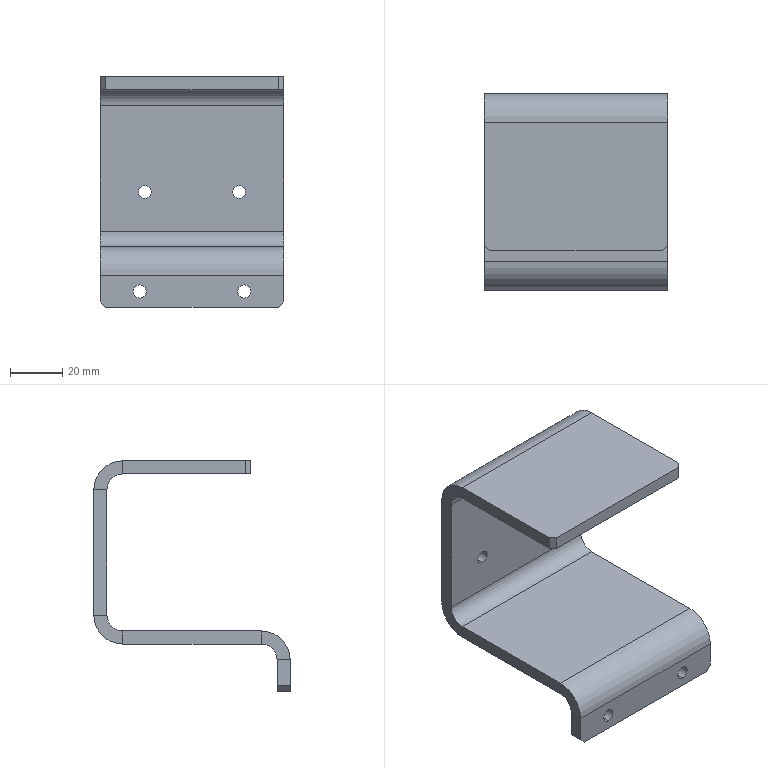Part | SolidWorks | features EdgeFlange 3, HoleWzd 2, Chamfer 1, FlatPattern 1, SMBaseFlange 1, SheetMetal 1 | 1 solid | 42 faces | box 70 x 75 x 88 mm | volume 70287 mm3 | plane 28 | cylinder 14 | commonest cylinder face diameters 5 x8 12 x3 22 x3
STEP:
#1=CARTESIAN_POINT('',(-20.,-45.,-84.5));
#2=VERTEX_POINT('',#1);
#3=CARTESIAN_POINT('',(-20.,-45.,-79.5));
#4=VERTEX_POINT('',#3);
#5=CARTESIAN_POINT('',(-20.,-45.,-82.));
#6=DIRECTION('',(0.,1.,0.));
#7=DIRECTION('',(0.,0.,1.));
#8=AXIS2_PLACEMENT_3D('',#5,#6,#7);
#9=CIRCLE('',#8,2.5);
#10=EDGE_CURVE('',#2,#4,#9,.T.);
#11=ORIENTED_EDGE('',*,*,#10,.F.);
#12=CARTESIAN_POINT('',(-20.,-40.,-84.5));
#13=VERTEX_POINT('',#12);
#14=CARTESIAN_POINT('',(-20.,-40.,-84.5));
#15=DIRECTION('',(0.,1.,0.));
#16=VECTOR('',#15,1000.);
#17=LINE('',#14,#16);
#18=EDGE_CURVE('',#2,#13,#17,.T.);
#19=ORIENTED_EDGE('',*,*,#18,.T.);
#20=CARTESIAN_POINT('',(-20.,-40.,-79.5));
#21=VERTEX_POINT('',#20);
#22=CARTESIAN_POINT('',(-20.,-40.,-82.));
#23=DIRECTION('',(0.,1.,0.));
#24=DIRECTION('',(0.,0.,1.));
#25=AXIS2_PLACEMENT_3D('',#22,#23,#24);
#26=CIRCLE('',#25,2.5);
#27=EDGE_CURVE('',#13,#21,#26,.T.);
#28=ORIENTED_EDGE('',*,*,#27,.T.);
#29=CARTESIAN_POINT('',(-20.,-40.,-79.5));
#30=DIRECTION('',(0.,1.,0.));
#31=VECTOR('',#30,1000.);
#32=LINE('',#29,#31);
#33=EDGE_CURVE('',#4,#21,#32,.T.);
#34=ORIENTED_EDGE('',*,*,#33,.F.);
#35=EDGE_LOOP('',(#11,#19,#28,#34));
#36=FACE_OUTER_BOUND('',#35,.T.);
#37=CARTESIAN_POINT('',(-20.,-40.,-82.));
#38=DIRECTION('',(0.,1.,0.));
#39=DIRECTION('',(0.,0.,1.));
#40=AXIS2_PLACEMENT_3D('',#37,#38,#39);
#41=CYLINDRICAL_SURFACE('',#40,2.5);
#42=ADVANCED_FACE('',(#36),#41,.F.);
#43=CARTESIAN_POINT('',(20.,-45.,-84.5));
#44=VERTEX_POINT('',#43);
#45=CARTESIAN_POINT('',(20.,-45.,-79.5));
#46=VERTEX_POINT('',#45);
#47=CARTESIAN_POINT('',(20.,-45.,-82.));
#48=DIRECTION('',(0.,1.,0.));
#49=DIRECTION('',(0.,0.,1.));
#50=AXIS2_PLACEMENT_3D('',#47,#48,#49);
#51=CIRCLE('',#50,2.5);
#52=EDGE_CURVE('',#44,#46,#51,.T.);
#53=ORIENTED_EDGE('',*,*,#52,.F.);
#54=CARTESIAN_POINT('',(20.,-40.,-84.5));
#55=VERTEX_POINT('',#54);
#56=CARTESIAN_POINT('',(20.,-40.,-84.5));
#57=DIRECTION('',(0.,1.,0.));
#58=VECTOR('',#57,1000.);
#59=LINE('',#56,#58);
#60=EDGE_CURVE('',#44,#55,#59,.T.);
#61=ORIENTED_EDGE('',*,*,#60,.T.);
#62=CARTESIAN_POINT('',(20.,-40.,-79.5));
#63=VERTEX_POINT('',#62);
#64=CARTESIAN_POINT('',(20.,-40.,-82.));
#65=DIRECTION('',(0.,1.,0.));
#66=DIRECTION('',(0.,0.,1.));
#67=AXIS2_PLACEMENT_3D('',#64,#65,#66);
#68=CIRCLE('',#67,2.5);
#69=EDGE_CURVE('',#55,#63,#68,.T.);
#70=ORIENTED_EDGE('',*,*,#69,.T.);
#71=CARTESIAN_POINT('',(20.,-40.,-79.5));
#72=DIRECTION('',(0.,1.,0.));
#73=VECTOR('',#72,1000.);
#74=LINE('',#71,#73);
#75=EDGE_CURVE('',#46,#63,#74,.T.);
#76=ORIENTED_EDGE('',*,*,#75,.F.);
#77=EDGE_LOOP('',(#53,#61,#70,#76));
#78=FACE_OUTER_BOUND('',#77,.T.);
#79=CARTESIAN_POINT('',(20.,-40.,-82.));
#80=DIRECTION('',(0.,1.,0.));
#81=DIRECTION('',(0.,0.,1.));
#82=AXIS2_PLACEMENT_3D('',#79,#80,#81);
#83=CYLINDRICAL_SURFACE('',#82,2.5);
#84=ADVANCED_FACE('',(#78),#83,.F.);
#85=CARTESIAN_POINT('',(-18.,25.,-46.5));
#86=VERTEX_POINT('',#85);
#87=CARTESIAN_POINT('',(-18.,25.,-41.5));
#88=VERTEX_POINT('',#87);
#89=CARTESIAN_POINT('',(-18.,25.,-44.));
#90=DIRECTION('',(0.,1.,0.));
#91=DIRECTION('',(0.,0.,1.));
#92=AXIS2_PLACEMENT_3D('',#89,#90,#91);
#93=CIRCLE('',#92,2.5);
#94=EDGE_CURVE('',#86,#88,#93,.T.);
#95=ORIENTED_EDGE('',*,*,#94,.F.);
#96=CARTESIAN_POINT('',(-18.,30.,-46.5));
#97=VERTEX_POINT('',#96);
#98=CARTESIAN_POINT('',(-18.,30.,-46.5));
#99=DIRECTION('',(0.,1.,0.));
#100=VECTOR('',#99,1000.);
#101=LINE('',#98,#100);
#102=EDGE_CURVE('',#86,#97,#101,.T.);
#103=ORIENTED_EDGE('',*,*,#102,.T.);
#104=CARTESIAN_POINT('',(-18.,30.,-41.5));
#105=VERTEX_POINT('',#104);
#106=CARTESIAN_POINT('',(-18.,30.,-44.));
#107=DIRECTION('',(0.,1.,0.));
#108=DIRECTION('',(0.,0.,1.));
#109=AXIS2_PLACEMENT_3D('',#106,#107,#108);
#110=CIRCLE('',#109,2.5);
#111=EDGE_CURVE('',#97,#105,#110,.T.);
#112=ORIENTED_EDGE('',*,*,#111,.T.);
#113=CARTESIAN_POINT('',(-18.,30.,-41.5));
#114=DIRECTION('',(0.,1.,0.));
#115=VECTOR('',#114,1000.);
#116=LINE('',#113,#115);
#117=EDGE_CURVE('',#88,#105,#116,.T.);
#118=ORIENTED_EDGE('',*,*,#117,.F.);
#119=EDGE_LOOP('',(#95,#103,#112,#118));
#120=FACE_OUTER_BOUND('',#119,.T.);
#121=CARTESIAN_POINT('',(-18.,30.,-44.));
#122=DIRECTION('',(0.,1.,0.));
#123=DIRECTION('',(0.,0.,1.));
#124=AXIS2_PLACEMENT_3D('',#121,#122,#123);
#125=CYLINDRICAL_SURFACE('',#124,2.5);
#126=ADVANCED_FACE('',(#120),#125,.F.);
#127=CARTESIAN_POINT('',(18.,25.,-46.5));
#128=VERTEX_POINT('',#127);
#129=CARTESIAN_POINT('',(18.,25.,-41.5));
#130=VERTEX_POINT('',#129);
#131=CARTESIAN_POINT('',(18.,25.,-44.));
#132=DIRECTION('',(0.,1.,0.));
#133=DIRECTION('',(0.,0.,1.));
#134=AXIS2_PLACEMENT_3D('',#131,#132,#133);
#135=CIRCLE('',#134,2.5);
#136=EDGE_CURVE('',#128,#130,#135,.T.);
#137=ORIENTED_EDGE('',*,*,#136,.F.);
#138=CARTESIAN_POINT('',(18.,30.,-46.5));
#139=VERTEX_POINT('',#138);
#140=CARTESIAN_POINT('',(18.,30.,-46.5));
#141=DIRECTION('',(0.,1.,0.));
#142=VECTOR('',#141,1000.);
#143=LINE('',#140,#142);
#144=EDGE_CURVE('',#128,#139,#143,.T.);
#145=ORIENTED_EDGE('',*,*,#144,.T.);
#146=CARTESIAN_POINT('',(18.,30.,-41.5));
#147=VERTEX_POINT('',#146);
#148=CARTESIAN_POINT('',(18.,30.,-44.));
#149=DIRECTION('',(0.,1.,0.));
#150=DIRECTION('',(0.,0.,1.));
#151=AXIS2_PLACEMENT_3D('',#148,#149,#150);
#152=CIRCLE('',#151,2.5);
#153=EDGE_CURVE('',#139,#147,#152,.T.);
#154=ORIENTED_EDGE('',*,*,#153,.T.);
#155=CARTESIAN_POINT('',(18.,30.,-41.5));
#156=DIRECTION('',(0.,1.,0.));
#157=VECTOR('',#156,1000.);
#158=LINE('',#155,#157);
#159=EDGE_CURVE('',#130,#147,#158,.T.);
#160=ORIENTED_EDGE('',*,*,#159,.F.);
#161=EDGE_LOOP('',(#137,#145,#154,#160));
#162=FACE_OUTER_BOUND('',#161,.T.);
#163=CARTESIAN_POINT('',(18.,30.,-44.));
#164=DIRECTION('',(0.,1.,0.));
#165=DIRECTION('',(0.,0.,1.));
#166=AXIS2_PLACEMENT_3D('',#163,#164,#165);
#167=CYLINDRICAL_SURFACE('',#166,2.5);
#168=ADVANCED_FACE('',(#162),#167,.F.);
#169=CARTESIAN_POINT('',(-35.,19.,-70.));
#170=VERTEX_POINT('',#169);
#171=CARTESIAN_POINT('',(-35.,-34.,-70.));
#172=VERTEX_POINT('',#171);
#173=CARTESIAN_POINT('',(-35.,-45.,-70.));
#174=DIRECTION('',(0.,-1.,0.));
#175=VECTOR('',#174,1000.);
#176=LINE('',#173,#175);
#177=EDGE_CURVE('',#170,#172,#176,.T.);
#178=ORIENTED_EDGE('',*,*,#177,.T.);
#179=CARTESIAN_POINT('',(-35.,-34.,-65.));
#180=VERTEX_POINT('',#179);
#181=CARTESIAN_POINT('',(-35.,-34.,-70.));
#182=DIRECTION('',(0.,0.,1.));
#183=VECTOR('',#182,1000.);
#184=LINE('',#181,#183);
#185=EDGE_CURVE('',#172,#180,#184,.T.);
#186=ORIENTED_EDGE('',*,*,#185,.T.);
#187=CARTESIAN_POINT('',(-35.,19.,-65.));
#188=VERTEX_POINT('',#187);
#189=CARTESIAN_POINT('',(-35.,0.,-65.));
#190=DIRECTION('',(0.,-1.,0.));
#191=VECTOR('',#190,1000.);
#192=LINE('',#189,#191);
#193=EDGE_CURVE('',#188,#180,#192,.T.);
#194=ORIENTED_EDGE('',*,*,#193,.F.);
#195=CARTESIAN_POINT('',(-35.,19.,-70.));
#196=DIRECTION('',(0.,0.,-1.));
#197=VECTOR('',#196,1000.);
#198=LINE('',#195,#197);
#199=EDGE_CURVE('',#188,#170,#198,.T.);
#200=ORIENTED_EDGE('',*,*,#199,.T.);
#201=EDGE_LOOP('',(#178,#186,#194,#200));
#202=FACE_OUTER_BOUND('',#201,.T.);
#203=CARTESIAN_POINT('',(-35.,-45.,-70.));
#204=DIRECTION('',(-1.,0.,0.));
#205=DIRECTION('',(0.,0.,1.));
#206=AXIS2_PLACEMENT_3D('',#203,#204,#205);
#207=PLANE('',#206);
#208=ADVANCED_FACE('',(#202),#207,.T.);
#209=CARTESIAN_POINT('',(35.,-34.,-70.));
#210=VERTEX_POINT('',#209);
#211=CARTESIAN_POINT('',(35.,19.,-70.));
#212=VERTEX_POINT('',#211);
#213=CARTESIAN_POINT('',(35.,25.,-70.));
#214=DIRECTION('',(0.,1.,0.));
#215=VECTOR('',#214,1000.);
#216=LINE('',#213,#215);
#217=EDGE_CURVE('',#210,#212,#216,.T.);
#218=ORIENTED_EDGE('',*,*,#217,.F.);
#219=CARTESIAN_POINT('',(-35.,-34.,-70.));
#220=DIRECTION('',(1.,0.,0.));
#221=VECTOR('',#220,1000.);
#222=LINE('',#219,#221);
#223=EDGE_CURVE('',#172,#210,#222,.T.);
#224=ORIENTED_EDGE('',*,*,#223,.F.);
#225=ORIENTED_EDGE('',*,*,#177,.F.);
#226=CARTESIAN_POINT('',(0.,19.,-70.));
#227=DIRECTION('',(1.,0.,0.));
#228=VECTOR('',#227,1000.);
#229=LINE('',#226,#228);
#230=EDGE_CURVE('',#170,#212,#229,.T.);
#231=ORIENTED_EDGE('',*,*,#230,.T.);
#232=EDGE_LOOP('',(#218,#224,#225,#231));
#233=FACE_OUTER_BOUND('',#232,.T.);
#234=CARTESIAN_POINT('',(0.,0.,-70.));
#235=DIRECTION('',(0.,0.,-1.));
#236=DIRECTION('',(0.,1.,0.));
#237=AXIS2_PLACEMENT_3D('',#234,#235,#236);
#238=PLANE('',#237);
#239=ADVANCED_FACE('',(#233),#238,.T.);
#240=CARTESIAN_POINT('',(35.,-34.,-65.));
#241=VERTEX_POINT('',#240);
#242=CARTESIAN_POINT('',(-35.,-34.,-65.));
#243=DIRECTION('',(1.,0.,0.));
#244=VECTOR('',#243,1000.);
#245=LINE('',#242,#244);
#246=EDGE_CURVE('',#180,#241,#245,.T.);
#247=ORIENTED_EDGE('',*,*,#246,.T.);
#248=CARTESIAN_POINT('',(35.,19.,-65.));
#249=VERTEX_POINT('',#248);
#250=CARTESIAN_POINT('',(35.,0.,-65.));
#251=DIRECTION('',(0.,1.,0.));
#252=VECTOR('',#251,1000.);
#253=LINE('',#250,#252);
#254=EDGE_CURVE('',#241,#249,#253,.T.);
#255=ORIENTED_EDGE('',*,*,#254,.T.);
#256=CARTESIAN_POINT('',(-35.,19.,-65.));
#257=DIRECTION('',(1.,0.,0.));
#258=VECTOR('',#257,1000.);
#259=LINE('',#256,#258);
#260=EDGE_CURVE('',#188,#249,#259,.T.);
#261=ORIENTED_EDGE('',*,*,#260,.F.);
#262=ORIENTED_EDGE('',*,*,#193,.T.);
#263=EDGE_LOOP('',(#247,#255,#261,#262));
#264=FACE_OUTER_BOUND('',#263,.T.);
#265=CARTESIAN_POINT('',(0.,0.,-65.));
#266=DIRECTION('',(0.,0.,-1.));
#267=DIRECTION('',(0.,1.,0.));
#268=AXIS2_PLACEMENT_3D('',#265,#266,#267);
#269=PLANE('',#268);
#270=ADVANCED_FACE('',(#264),#269,.F.);
#271=CARTESIAN_POINT('',(35.,25.,-59.));
#272=VERTEX_POINT('',#271);
#273=CARTESIAN_POINT('',(35.,25.,-11.));
#274=VERTEX_POINT('',#273);
#275=CARTESIAN_POINT('',(35.,25.,0.));
#276=DIRECTION('',(0.,0.,1.));
#277=VECTOR('',#276,1000.);
#278=LINE('',#275,#277);
#279=EDGE_CURVE('',#272,#274,#278,.T.);
#280=ORIENTED_EDGE('',*,*,#279,.F.);
#281=CARTESIAN_POINT('',(35.,30.,-59.));
#282=VERTEX_POINT('',#281);
#283=CARTESIAN_POINT('',(35.,25.,-59.));
#284=DIRECTION('',(0.,1.,0.));
#285=VECTOR('',#284,1000.);
#286=LINE('',#283,#285);
#287=EDGE_CURVE('',#272,#282,#286,.T.);
#288=ORIENTED_EDGE('',*,*,#287,.T.);
#289=CARTESIAN_POINT('',(35.,30.,-11.));
#290=VERTEX_POINT('',#289);
#291=CARTESIAN_POINT('',(35.,30.,-5.));
#292=DIRECTION('',(0.,0.,1.));
#293=VECTOR('',#292,1000.);
#294=LINE('',#291,#293);
#295=EDGE_CURVE('',#282,#290,#294,.T.);
#296=ORIENTED_EDGE('',*,*,#295,.T.);
#297=CARTESIAN_POINT('',(35.,25.,-11.));
#298=DIRECTION('',(0.,1.,0.));
#299=VECTOR('',#298,1000.);
#300=LINE('',#297,#299);
#301=EDGE_CURVE('',#274,#290,#300,.T.);
#302=ORIENTED_EDGE('',*,*,#301,.F.);
#303=EDGE_LOOP('',(#280,#288,#296,#302));
#304=FACE_OUTER_BOUND('',#303,.T.);
#305=CARTESIAN_POINT('',(35.,30.,-5.));
#306=DIRECTION('',(1.,0.,0.));
#307=DIRECTION('',(0.,0.,-1.));
#308=AXIS2_PLACEMENT_3D('',#305,#306,#307);
#309=PLANE('',#308);
#310=ADVANCED_FACE('',(#304),#309,.T.);
#311=CARTESIAN_POINT('',(-18.,30.,-44.));
#312=DIRECTION('',(0.,1.,0.));
#313=DIRECTION('',(0.,0.,1.));
#314=AXIS2_PLACEMENT_3D('',#311,#312,#313);
#315=CIRCLE('',#314,2.5);
#316=EDGE_CURVE('',#105,#97,#315,.T.);
#317=ORIENTED_EDGE('',*,*,#316,.F.);
#318=ORIENTED_EDGE('',*,*,#111,.F.);
#319=EDGE_LOOP('',(#317,#318));
#320=FACE_BOUND('',#319,.T.);
#321=CARTESIAN_POINT('',(18.,30.,-44.));
#322=DIRECTION('',(0.,1.,0.));
#323=DIRECTION('',(0.,0.,1.));
#324=AXIS2_PLACEMENT_3D('',#321,#322,#323);
#325=CIRCLE('',#324,2.5);
#326=EDGE_CURVE('',#147,#139,#325,.T.);
#327=ORIENTED_EDGE('',*,*,#326,.F.);
#328=ORIENTED_EDGE('',*,*,#153,.F.);
#329=EDGE_LOOP('',(#327,#328));
#330=FACE_BOUND('',#329,.T.);
#331=ORIENTED_EDGE('',*,*,#295,.F.);
#332=CARTESIAN_POINT('',(-35.,30.,-59.));
#333=VERTEX_POINT('',#332);
#334=CARTESIAN_POINT('',(35.,30.,-59.));
#335=DIRECTION('',(-1.,0.,0.));
#336=VECTOR('',#335,1000.);
#337=LINE('',#334,#336);
#338=EDGE_CURVE('',#282,#333,#337,.T.);
#339=ORIENTED_EDGE('',*,*,#338,.T.);
#340=CARTESIAN_POINT('',(-35.,30.,-11.));
#341=VERTEX_POINT('',#340);
#342=CARTESIAN_POINT('',(-35.,30.,-70.));
#343=DIRECTION('',(0.,0.,-1.));
#344=VECTOR('',#343,1000.);
#345=LINE('',#342,#344);
#346=EDGE_CURVE('',#341,#333,#345,.T.);
#347=ORIENTED_EDGE('',*,*,#346,.F.);
#348=CARTESIAN_POINT('',(0.,30.,-11.));
#349=DIRECTION('',(1.,0.,0.));
#350=VECTOR('',#349,1000.);
#351=LINE('',#348,#350);
#352=EDGE_CURVE('',#341,#290,#351,.T.);
#353=ORIENTED_EDGE('',*,*,#352,.T.);
#354=EDGE_LOOP('',(#331,#339,#347,#353));
#355=FACE_OUTER_BOUND('',#354,.T.);
#356=CARTESIAN_POINT('',(0.,30.,0.));
#357=DIRECTION('',(0.,1.,0.));
#358=DIRECTION('',(0.,0.,1.));
#359=AXIS2_PLACEMENT_3D('',#356,#357,#358);
#360=PLANE('',#359);
#361=ADVANCED_FACE('',(#320,#330,#355),#360,.T.);
#362=CARTESIAN_POINT('',(-18.,25.,-44.));
#363=DIRECTION('',(0.,1.,0.));
#364=DIRECTION('',(0.,0.,1.));
#365=AXIS2_PLACEMENT_3D('',#362,#363,#364);
#366=CIRCLE('',#365,2.5);
#367=EDGE_CURVE('',#88,#86,#366,.T.);
#368=ORIENTED_EDGE('',*,*,#367,.T.);
#369=ORIENTED_EDGE('',*,*,#94,.T.);
#370=EDGE_LOOP('',(#368,#369));
#371=FACE_BOUND('',#370,.T.);
#372=CARTESIAN_POINT('',(18.,25.,-44.));
#373=DIRECTION('',(0.,1.,0.));
#374=DIRECTION('',(0.,0.,1.));
#375=AXIS2_PLACEMENT_3D('',#372,#373,#374);
#376=CIRCLE('',#375,2.5);
#377=EDGE_CURVE('',#130,#128,#376,.T.);
#378=ORIENTED_EDGE('',*,*,#377,.T.);
#379=ORIENTED_EDGE('',*,*,#136,.T.);
#380=EDGE_LOOP('',(#378,#379));
#381=FACE_BOUND('',#380,.T.);
#382=CARTESIAN_POINT('',(-35.,25.,-59.));
#383=VERTEX_POINT('',#382);
#384=CARTESIAN_POINT('',(35.,25.,-59.));
#385=DIRECTION('',(-1.,0.,0.));
#386=VECTOR('',#385,1000.);
#387=LINE('',#384,#386);
#388=EDGE_CURVE('',#272,#383,#387,.T.);
#389=ORIENTED_EDGE('',*,*,#388,.F.);
#390=ORIENTED_EDGE('',*,*,#279,.T.);
#391=CARTESIAN_POINT('',(-35.,25.,-11.));
#392=VERTEX_POINT('',#391);
#393=CARTESIAN_POINT('',(-35.,25.,-11.));
#394=DIRECTION('',(1.,0.,0.));
#395=VECTOR('',#394,1000.);
#396=LINE('',#393,#395);
#397=EDGE_CURVE('',#392,#274,#396,.T.);
#398=ORIENTED_EDGE('',*,*,#397,.F.);
#399=CARTESIAN_POINT('',(-35.,25.,0.));
#400=DIRECTION('',(0.,0.,-1.));
#401=VECTOR('',#400,1000.);
#402=LINE('',#399,#401);
#403=EDGE_CURVE('',#392,#383,#402,.T.);
#404=ORIENTED_EDGE('',*,*,#403,.T.);
#405=EDGE_LOOP('',(#389,#390,#398,#404));
#406=FACE_OUTER_BOUND('',#405,.T.);
#407=CARTESIAN_POINT('',(0.,25.,0.));
#408=DIRECTION('',(0.,1.,0.));
#409=DIRECTION('',(0.,0.,1.));
#410=AXIS2_PLACEMENT_3D('',#407,#408,#409);
#411=PLANE('',#410);
#412=ADVANCED_FACE('',(#371,#381,#406),#411,.F.);
#413=CARTESIAN_POINT('',(35.,-28.,0.));
#414=VERTEX_POINT('',#413);
#415=CARTESIAN_POINT('',(35.,19.,0.));
#416=VERTEX_POINT('',#415);
#417=CARTESIAN_POINT('',(35.,-30.,0.));
#418=DIRECTION('',(0.,1.,0.));
#419=VECTOR('',#418,1000.);
#420=LINE('',#417,#419);
#421=EDGE_CURVE('',#414,#416,#420,.T.);
#422=ORIENTED_EDGE('',*,*,#421,.F.);
#423=CARTESIAN_POINT('',(35.,-28.,-5.));
#424=VERTEX_POINT('',#423);
#425=CARTESIAN_POINT('',(35.,-28.,-5.));
#426=DIRECTION('',(0.,0.,-1.));
#427=VECTOR('',#426,1000.);
#428=LINE('',#425,#427);
#429=EDGE_CURVE('',#414,#424,#428,.T.);
#430=ORIENTED_EDGE('',*,*,#429,.T.);
#431=CARTESIAN_POINT('',(35.,19.,-5.));
#432=VERTEX_POINT('',#431);
#433=CARTESIAN_POINT('',(35.,-30.,-5.));
#434=DIRECTION('',(0.,1.,0.));
#435=VECTOR('',#434,1000.);
#436=LINE('',#433,#435);
#437=EDGE_CURVE('',#424,#432,#436,.T.);
#438=ORIENTED_EDGE('',*,*,#437,.T.);
#439=CARTESIAN_POINT('',(35.,19.,-5.));
#440=DIRECTION('',(0.,0.,1.));
#441=VECTOR('',#440,1000.);
#442=LINE('',#439,#441);
#443=EDGE_CURVE('',#432,#416,#442,.T.);
#444=ORIENTED_EDGE('',*,*,#443,.T.);
#445=EDGE_LOOP('',(#422,#430,#438,#444));
#446=FACE_OUTER_BOUND('',#445,.T.);
#447=CARTESIAN_POINT('',(35.,-30.,-5.));
#448=DIRECTION('',(1.,0.,0.));
#449=DIRECTION('',(0.,0.,-1.));
#450=AXIS2_PLACEMENT_3D('',#447,#448,#449);
#451=PLANE('',#450);
#452=ADVANCED_FACE('',(#446),#451,.T.);
#453=ORIENTED_EDGE('',*,*,#437,.F.);
#454=CARTESIAN_POINT('',(33.,-30.,-5.));
#455=VERTEX_POINT('',#454);
#456=CARTESIAN_POINT('',(31.5,-31.5,-5.));
#457=DIRECTION('',(-0.7071,-0.7071,0.));
#458=VECTOR('',#457,1000.);
#459=LINE('',#456,#458);
#460=EDGE_CURVE('',#424,#455,#459,.T.);
#461=ORIENTED_EDGE('',*,*,#460,.T.);
#462=CARTESIAN_POINT('',(-33.,-30.,-5.));
#463=VERTEX_POINT('',#462);
#464=CARTESIAN_POINT('',(-35.,-30.,-5.));
#465=DIRECTION('',(1.,0.,0.));
#466=VECTOR('',#465,1000.);
#467=LINE('',#464,#466);
#468=EDGE_CURVE('',#463,#455,#467,.T.);
#469=ORIENTED_EDGE('',*,*,#468,.F.);
#470=CARTESIAN_POINT('',(-35.,-28.,-5.));
#471=VERTEX_POINT('',#470);
#472=CARTESIAN_POINT('',(-31.5,-31.5,-5.));
#473=DIRECTION('',(-0.7071,0.7071,0.));
#474=VECTOR('',#473,1000.);
#475=LINE('',#472,#474);
#476=EDGE_CURVE('',#463,#471,#475,.T.);
#477=ORIENTED_EDGE('',*,*,#476,.T.);
#478=CARTESIAN_POINT('',(-35.,19.,-5.));
#479=VERTEX_POINT('',#478);
#480=CARTESIAN_POINT('',(-35.,-30.,-5.));
#481=DIRECTION('',(0.,-1.,0.));
#482=VECTOR('',#481,1000.);
#483=LINE('',#480,#482);
#484=EDGE_CURVE('',#479,#471,#483,.T.);
#485=ORIENTED_EDGE('',*,*,#484,.F.);
#486=CARTESIAN_POINT('',(35.,19.,-5.));
#487=DIRECTION('',(-1.,0.,0.));
#488=VECTOR('',#487,1000.);
#489=LINE('',#486,#488);
#490=EDGE_CURVE('',#432,#479,#489,.T.);
#491=ORIENTED_EDGE('',*,*,#490,.F.);
#492=EDGE_LOOP('',(#453,#461,#469,#477,#485,#491));
#493=FACE_OUTER_BOUND('',#492,.T.);
#494=CARTESIAN_POINT('',(0.,0.,-5.));
#495=DIRECTION('',(0.,0.,-1.));
#496=DIRECTION('',(-1.,0.,0.));
#497=AXIS2_PLACEMENT_3D('',#494,#495,#496);
#498=PLANE('',#497);
#499=ADVANCED_FACE('',(#493),#498,.T.);
#500=CARTESIAN_POINT('',(-33.,-30.,0.));
#501=VERTEX_POINT('',#500);
#502=CARTESIAN_POINT('',(33.,-30.,0.));
#503=VERTEX_POINT('',#502);
#504=CARTESIAN_POINT('',(-35.,-30.,0.));
#505=DIRECTION('',(1.,0.,0.));
#506=VECTOR('',#505,1000.);
#507=LINE('',#504,#506);
#508=EDGE_CURVE('',#501,#503,#507,.T.);
#509=ORIENTED_EDGE('',*,*,#508,.T.);
#510=CARTESIAN_POINT('',(33.,-30.,0.));
#511=DIRECTION('',(0.7071,0.7071,0.));
#512=VECTOR('',#511,1000.);
#513=LINE('',#510,#512);
#514=EDGE_CURVE('',#503,#414,#513,.T.);
#515=ORIENTED_EDGE('',*,*,#514,.T.);
#516=ORIENTED_EDGE('',*,*,#421,.T.);
#517=CARTESIAN_POINT('',(-35.,19.,0.));
#518=VERTEX_POINT('',#517);
#519=CARTESIAN_POINT('',(35.,19.,0.));
#520=DIRECTION('',(-1.,0.,0.));
#521=VECTOR('',#520,1000.);
#522=LINE('',#519,#521);
#523=EDGE_CURVE('',#416,#518,#522,.T.);
#524=ORIENTED_EDGE('',*,*,#523,.T.);
#525=CARTESIAN_POINT('',(-35.,-28.,0.));
#526=VERTEX_POINT('',#525);
#527=CARTESIAN_POINT('',(-35.,-30.,0.));
#528=DIRECTION('',(0.,-1.,0.));
#529=VECTOR('',#528,1000.);
#530=LINE('',#527,#529);
#531=EDGE_CURVE('',#518,#526,#530,.T.);
#532=ORIENTED_EDGE('',*,*,#531,.T.);
#533=CARTESIAN_POINT('',(-35.,-28.,0.));
#534=DIRECTION('',(0.7071,-0.7071,0.));
#535=VECTOR('',#534,1000.);
#536=LINE('',#533,#535);
#537=EDGE_CURVE('',#526,#501,#536,.T.);
#538=ORIENTED_EDGE('',*,*,#537,.T.);
#539=EDGE_LOOP('',(#509,#515,#516,#524,#532,#538));
#540=FACE_OUTER_BOUND('',#539,.T.);
#541=CARTESIAN_POINT('',(0.,0.,0.));
#542=DIRECTION('',(0.,0.,-1.));
#543=DIRECTION('',(-1.,0.,0.));
#544=AXIS2_PLACEMENT_3D('',#541,#542,#543);
#545=PLANE('',#544);
#546=ADVANCED_FACE('',(#540),#545,.F.);
#547=ORIENTED_EDGE('',*,*,#468,.T.);
#548=CARTESIAN_POINT('',(33.,-30.,-5.));
#549=DIRECTION('',(0.,0.,1.));
#550=VECTOR('',#549,1000.);
#551=LINE('',#548,#550);
#552=EDGE_CURVE('',#455,#503,#551,.T.);
#553=ORIENTED_EDGE('',*,*,#552,.T.);
#554=ORIENTED_EDGE('',*,*,#508,.F.);
#555=CARTESIAN_POINT('',(-33.,-30.,-5.));
#556=DIRECTION('',(0.,0.,-1.));
#557=VECTOR('',#556,1000.);
#558=LINE('',#555,#557);
#559=EDGE_CURVE('',#501,#463,#558,.T.);
#560=ORIENTED_EDGE('',*,*,#559,.T.);
#561=EDGE_LOOP('',(#547,#553,#554,#560));
#562=FACE_OUTER_BOUND('',#561,.T.);
#563=CARTESIAN_POINT('',(-35.,-30.,-5.));
#564=DIRECTION('',(0.,-1.,0.));
#565=DIRECTION('',(0.,0.,-1.));
#566=AXIS2_PLACEMENT_3D('',#563,#564,#565);
#567=PLANE('',#566);
#568=ADVANCED_FACE('',(#562),#567,.T.);
#569=ORIENTED_EDGE('',*,*,#484,.T.);
#570=CARTESIAN_POINT('',(-35.,-28.,-5.));
#571=DIRECTION('',(0.,0.,1.));
#572=VECTOR('',#571,1000.);
#573=LINE('',#570,#572);
#574=EDGE_CURVE('',#471,#526,#573,.T.);
#575=ORIENTED_EDGE('',*,*,#574,.T.);
#576=ORIENTED_EDGE('',*,*,#531,.F.);
#577=CARTESIAN_POINT('',(-35.,19.,-5.));
#578=DIRECTION('',(0.,0.,1.));
#579=VECTOR('',#578,1000.);
#580=LINE('',#577,#579);
#581=EDGE_CURVE('',#479,#518,#580,.T.);
#582=ORIENTED_EDGE('',*,*,#581,.F.);
#583=EDGE_LOOP('',(#569,#575,#576,#582));
#584=FACE_OUTER_BOUND('',#583,.T.);
#585=CARTESIAN_POINT('',(-35.,-30.,-5.));
#586=DIRECTION('',(-1.,0.,0.));
#587=DIRECTION('',(0.,0.,1.));
#588=AXIS2_PLACEMENT_3D('',#585,#586,#587);
#589=PLANE('',#588);
#590=ADVANCED_FACE('',(#584),#589,.T.);
#591=CARTESIAN_POINT('',(-35.,30.,-11.));
#592=DIRECTION('',(0.,1.,0.));
#593=VECTOR('',#592,1000.);
#594=LINE('',#591,#593);
#595=EDGE_CURVE('',#392,#341,#594,.T.);
#596=ORIENTED_EDGE('',*,*,#595,.F.);
#597=CARTESIAN_POINT('',(-35.,19.,-11.));
#598=DIRECTION('',(-1.,0.,0.));
#599=DIRECTION('',(0.,0.,-1.));
#600=AXIS2_PLACEMENT_3D('',#597,#598,#599);
#601=CIRCLE('',#600,6.);
#602=EDGE_CURVE('',#479,#392,#601,.T.);
#603=ORIENTED_EDGE('',*,*,#602,.F.);
#604=ORIENTED_EDGE('',*,*,#581,.T.);
#605=CARTESIAN_POINT('',(-35.,19.,-11.));
#606=DIRECTION('',(-1.,0.,0.));
#607=DIRECTION('',(0.,0.,-1.));
#608=AXIS2_PLACEMENT_3D('',#605,#606,#607);
#609=CIRCLE('',#608,11.);
#610=EDGE_CURVE('',#518,#341,#609,.T.);
#611=ORIENTED_EDGE('',*,*,#610,.T.);
#612=EDGE_LOOP('',(#596,#603,#604,#611));
#613=FACE_OUTER_BOUND('',#612,.T.);
#614=CARTESIAN_POINT('',(-35.,19.,-11.));
#615=DIRECTION('',(-1.,0.,0.));
#616=DIRECTION('',(0.,0.,1.));
#617=AXIS2_PLACEMENT_3D('',#614,#615,#616);
#618=PLANE('',#617);
#619=ADVANCED_FACE('',(#613),#618,.T.);
#620=CARTESIAN_POINT('',(35.,19.,-11.));
#621=DIRECTION('',(1.,0.,0.));
#622=DIRECTION('',(0.,0.,-1.));
#623=AXIS2_PLACEMENT_3D('',#620,#621,#622);
#624=CIRCLE('',#623,6.);
#625=EDGE_CURVE('',#274,#432,#624,.T.);
#626=ORIENTED_EDGE('',*,*,#625,.F.);
#627=ORIENTED_EDGE('',*,*,#301,.T.);
#628=CARTESIAN_POINT('',(35.,19.,-11.));
#629=DIRECTION('',(1.,0.,0.));
#630=DIRECTION('',(0.,0.,-1.));
#631=AXIS2_PLACEMENT_3D('',#628,#629,#630);
#632=CIRCLE('',#631,11.);
#633=EDGE_CURVE('',#290,#416,#632,.T.);
#634=ORIENTED_EDGE('',*,*,#633,.T.);
#635=ORIENTED_EDGE('',*,*,#443,.F.);
#636=EDGE_LOOP('',(#626,#627,#634,#635));
#637=FACE_OUTER_BOUND('',#636,.T.);
#638=CARTESIAN_POINT('',(35.,19.,-11.));
#639=DIRECTION('',(-1.,0.,0.));
#640=DIRECTION('',(0.,0.,1.));
#641=AXIS2_PLACEMENT_3D('',#638,#639,#640);
#642=PLANE('',#641);
#643=ADVANCED_FACE('',(#637),#642,.F.);
#644=ORIENTED_EDGE('',*,*,#523,.F.);
#645=ORIENTED_EDGE('',*,*,#633,.F.);
#646=ORIENTED_EDGE('',*,*,#352,.F.);
#647=ORIENTED_EDGE('',*,*,#610,.F.);
#648=EDGE_LOOP('',(#644,#645,#646,#647));
#649=FACE_OUTER_BOUND('',#648,.T.);
#650=CARTESIAN_POINT('',(35.,19.,-11.));
#651=DIRECTION('',(1.,0.,0.));
#652=DIRECTION('',(0.,1.,0.));
#653=AXIS2_PLACEMENT_3D('',#650,#651,#652);
#654=CYLINDRICAL_SURFACE('',#653,11.);
#655=ADVANCED_FACE('',(#649),#654,.T.);
#656=ORIENTED_EDGE('',*,*,#490,.T.);
#657=ORIENTED_EDGE('',*,*,#602,.T.);
#658=ORIENTED_EDGE('',*,*,#397,.T.);
#659=ORIENTED_EDGE('',*,*,#625,.T.);
#660=EDGE_LOOP('',(#656,#657,#658,#659));
#661=FACE_OUTER_BOUND('',#660,.T.);
#662=CARTESIAN_POINT('',(35.,19.,-11.));
#663=DIRECTION('',(1.,0.,0.));
#664=DIRECTION('',(0.,1.,0.));
#665=AXIS2_PLACEMENT_3D('',#662,#663,#664);
#666=CYLINDRICAL_SURFACE('',#665,6.);
#667=ADVANCED_FACE('',(#661),#666,.F.);
#668=CARTESIAN_POINT('',(-35.,25.,-59.));
#669=DIRECTION('',(0.,1.,0.));
#670=VECTOR('',#669,1000.);
#671=LINE('',#668,#670);
#672=EDGE_CURVE('',#383,#333,#671,.T.);
#673=ORIENTED_EDGE('',*,*,#672,.F.);
#674=ORIENTED_EDGE('',*,*,#403,.F.);
#675=ORIENTED_EDGE('',*,*,#595,.T.);
#676=ORIENTED_EDGE('',*,*,#346,.T.);
#677=EDGE_LOOP('',(#673,#674,#675,#676));
#678=FACE_OUTER_BOUND('',#677,.T.);
#679=CARTESIAN_POINT('',(-35.,30.,-70.));
#680=DIRECTION('',(-1.,0.,0.));
#681=DIRECTION('',(0.,0.,1.));
#682=AXIS2_PLACEMENT_3D('',#679,#680,#681);
#683=PLANE('',#682);
#684=ADVANCED_FACE('',(#678),#683,.T.);
#685=ORIENTED_EDGE('',*,*,#199,.F.);
#686=CARTESIAN_POINT('',(-35.,19.,-59.));
#687=DIRECTION('',(-1.,0.,0.));
#688=DIRECTION('',(0.,0.,-1.));
#689=AXIS2_PLACEMENT_3D('',#686,#687,#688);
#690=CIRCLE('',#689,6.);
#691=EDGE_CURVE('',#383,#188,#690,.T.);
#692=ORIENTED_EDGE('',*,*,#691,.F.);
#693=ORIENTED_EDGE('',*,*,#672,.T.);
#694=CARTESIAN_POINT('',(-35.,19.,-59.));
#695=DIRECTION('',(-1.,0.,0.));
#696=DIRECTION('',(0.,0.,-1.));
#697=AXIS2_PLACEMENT_3D('',#694,#695,#696);
#698=CIRCLE('',#697,11.);
#699=EDGE_CURVE('',#333,#170,#698,.T.);
#700=ORIENTED_EDGE('',*,*,#699,.T.);
#701=EDGE_LOOP('',(#685,#692,#693,#700));
#702=FACE_OUTER_BOUND('',#701,.T.);
#703=CARTESIAN_POINT('',(-35.,19.,-59.));
#704=DIRECTION('',(-1.,0.,0.));
#705=DIRECTION('',(0.,0.,1.));
#706=AXIS2_PLACEMENT_3D('',#703,#704,#705);
#707=PLANE('',#706);
#708=ADVANCED_FACE('',(#702),#707,.T.);
#709=CARTESIAN_POINT('',(35.,19.,-59.));
#710=DIRECTION('',(1.,0.,0.));
#711=DIRECTION('',(0.,0.,-1.));
#712=AXIS2_PLACEMENT_3D('',#709,#710,#711);
#713=CIRCLE('',#712,6.);
#714=EDGE_CURVE('',#249,#272,#713,.T.);
#715=ORIENTED_EDGE('',*,*,#714,.F.);
#716=CARTESIAN_POINT('',(35.,19.,-65.));
#717=DIRECTION('',(0.,0.,-1.));
#718=VECTOR('',#717,1000.);
#719=LINE('',#716,#718);
#720=EDGE_CURVE('',#249,#212,#719,.T.);
#721=ORIENTED_EDGE('',*,*,#720,.T.);
#722=CARTESIAN_POINT('',(35.,19.,-59.));
#723=DIRECTION('',(1.,0.,0.));
#724=DIRECTION('',(0.,0.,-1.));
#725=AXIS2_PLACEMENT_3D('',#722,#723,#724);
#726=CIRCLE('',#725,11.);
#727=EDGE_CURVE('',#212,#282,#726,.T.);
#728=ORIENTED_EDGE('',*,*,#727,.T.);
#729=ORIENTED_EDGE('',*,*,#287,.F.);
#730=EDGE_LOOP('',(#715,#721,#728,#729));
#731=FACE_OUTER_BOUND('',#730,.T.);
#732=CARTESIAN_POINT('',(35.,19.,-59.));
#733=DIRECTION('',(-1.,0.,0.));
#734=DIRECTION('',(0.,0.,1.));
#735=AXIS2_PLACEMENT_3D('',#732,#733,#734);
#736=PLANE('',#735);
#737=ADVANCED_FACE('',(#731),#736,.F.);
#738=ORIENTED_EDGE('',*,*,#338,.F.);
#739=ORIENTED_EDGE('',*,*,#727,.F.);
#740=ORIENTED_EDGE('',*,*,#230,.F.);
#741=ORIENTED_EDGE('',*,*,#699,.F.);
#742=EDGE_LOOP('',(#738,#739,#740,#741));
#743=FACE_OUTER_BOUND('',#742,.T.);
#744=CARTESIAN_POINT('',(35.,19.,-59.));
#745=DIRECTION('',(1.,0.,0.));
#746=DIRECTION('',(0.,0.,-1.));
#747=AXIS2_PLACEMENT_3D('',#744,#745,#746);
#748=CYLINDRICAL_SURFACE('',#747,11.);
#749=ADVANCED_FACE('',(#743),#748,.T.);
#750=ORIENTED_EDGE('',*,*,#388,.T.);
#751=ORIENTED_EDGE('',*,*,#691,.T.);
#752=ORIENTED_EDGE('',*,*,#260,.T.);
#753=ORIENTED_EDGE('',*,*,#714,.T.);
#754=EDGE_LOOP('',(#750,#751,#752,#753));
#755=FACE_OUTER_BOUND('',#754,.T.);
#756=CARTESIAN_POINT('',(35.,19.,-59.));
#757=DIRECTION('',(1.,0.,0.));
#758=DIRECTION('',(0.,0.,-1.));
#759=AXIS2_PLACEMENT_3D('',#756,#757,#758);
#760=CYLINDRICAL_SURFACE('',#759,6.);
#761=ADVANCED_FACE('',(#755),#760,.F.);
#762=CARTESIAN_POINT('',(35.,-34.,-70.));
#763=DIRECTION('',(0.,0.,1.));
#764=VECTOR('',#763,1000.);
#765=LINE('',#762,#764);
#766=EDGE_CURVE('',#210,#241,#765,.T.);
#767=ORIENTED_EDGE('',*,*,#766,.F.);
#768=ORIENTED_EDGE('',*,*,#217,.T.);
#769=ORIENTED_EDGE('',*,*,#720,.F.);
#770=ORIENTED_EDGE('',*,*,#254,.F.);
#771=EDGE_LOOP('',(#767,#768,#769,#770));
#772=FACE_OUTER_BOUND('',#771,.T.);
#773=CARTESIAN_POINT('',(35.,25.,-70.));
#774=DIRECTION('',(1.,0.,0.));
#775=DIRECTION('',(0.,0.,-1.));
#776=AXIS2_PLACEMENT_3D('',#773,#774,#775);
#777=PLANE('',#776);
#778=ADVANCED_FACE('',(#772),#777,.T.);
#779=CARTESIAN_POINT('',(35.,-40.,-76.));
#780=VERTEX_POINT('',#779);
#781=CARTESIAN_POINT('',(35.,-45.,-76.));
#782=VERTEX_POINT('',#781);
#783=CARTESIAN_POINT('',(35.,-45.,-76.));
#784=DIRECTION('',(0.,-1.,0.));
#785=VECTOR('',#784,1000.);
#786=LINE('',#783,#785);
#787=EDGE_CURVE('',#780,#782,#786,.T.);
#788=ORIENTED_EDGE('',*,*,#787,.F.);
#789=CARTESIAN_POINT('',(35.,-34.,-76.));
#790=DIRECTION('',(1.,0.,0.));
#791=DIRECTION('',(0.,0.,1.));
#792=AXIS2_PLACEMENT_3D('',#789,#790,#791);
#793=CIRCLE('',#792,6.);
#794=EDGE_CURVE('',#210,#780,#793,.T.);
#795=ORIENTED_EDGE('',*,*,#794,.F.);
#796=ORIENTED_EDGE('',*,*,#766,.T.);
#797=CARTESIAN_POINT('',(35.,-34.,-76.));
#798=DIRECTION('',(1.,0.,0.));
#799=DIRECTION('',(0.,0.,1.));
#800=AXIS2_PLACEMENT_3D('',#797,#798,#799);
#801=CIRCLE('',#800,11.);
#802=EDGE_CURVE('',#241,#782,#801,.T.);
#803=ORIENTED_EDGE('',*,*,#802,.T.);
#804=EDGE_LOOP('',(#788,#795,#796,#803));
#805=FACE_OUTER_BOUND('',#804,.T.);
#806=CARTESIAN_POINT('',(35.,-34.,-76.));
#807=DIRECTION('',(1.,0.,0.));
#808=DIRECTION('',(0.,0.,-1.));
#809=AXIS2_PLACEMENT_3D('',#806,#807,#808);
#810=PLANE('',#809);
#811=ADVANCED_FACE('',(#805),#810,.T.);
#812=CARTESIAN_POINT('',(-35.,-40.,-76.));
#813=VERTEX_POINT('',#812);
#814=CARTESIAN_POINT('',(-35.,-34.,-76.));
#815=DIRECTION('',(-1.,0.,0.));
#816=DIRECTION('',(0.,0.,1.));
#817=AXIS2_PLACEMENT_3D('',#814,#815,#816);
#818=CIRCLE('',#817,6.);
#819=EDGE_CURVE('',#813,#172,#818,.T.);
#820=ORIENTED_EDGE('',*,*,#819,.F.);
#821=CARTESIAN_POINT('',(-35.,-45.,-76.));
#822=VERTEX_POINT('',#821);
#823=CARTESIAN_POINT('',(-35.,-40.,-76.));
#824=DIRECTION('',(0.,-1.,0.));
#825=VECTOR('',#824,1000.);
#826=LINE('',#823,#825);
#827=EDGE_CURVE('',#813,#822,#826,.T.);
#828=ORIENTED_EDGE('',*,*,#827,.T.);
#829=CARTESIAN_POINT('',(-35.,-34.,-76.));
#830=DIRECTION('',(-1.,0.,0.));
#831=DIRECTION('',(0.,0.,1.));
#832=AXIS2_PLACEMENT_3D('',#829,#830,#831);
#833=CIRCLE('',#832,11.);
#834=EDGE_CURVE('',#822,#180,#833,.T.);
#835=ORIENTED_EDGE('',*,*,#834,.T.);
#836=ORIENTED_EDGE('',*,*,#185,.F.);
#837=EDGE_LOOP('',(#820,#828,#835,#836));
#838=FACE_OUTER_BOUND('',#837,.T.);
#839=CARTESIAN_POINT('',(-35.,-34.,-76.));
#840=DIRECTION('',(1.,0.,0.));
#841=DIRECTION('',(0.,0.,-1.));
#842=AXIS2_PLACEMENT_3D('',#839,#840,#841);
#843=PLANE('',#842);
#844=ADVANCED_FACE('',(#838),#843,.F.);
#845=ORIENTED_EDGE('',*,*,#246,.F.);
#846=ORIENTED_EDGE('',*,*,#834,.F.);
#847=CARTESIAN_POINT('',(0.,-45.,-76.));
#848=DIRECTION('',(-1.,0.,0.));
#849=VECTOR('',#848,1000.);
#850=LINE('',#847,#849);
#851=EDGE_CURVE('',#782,#822,#850,.T.);
#852=ORIENTED_EDGE('',*,*,#851,.F.);
#853=ORIENTED_EDGE('',*,*,#802,.F.);
#854=EDGE_LOOP('',(#845,#846,#852,#853));
#855=FACE_OUTER_BOUND('',#854,.T.);
#856=CARTESIAN_POINT('',(-35.,-34.,-76.));
#857=DIRECTION('',(-1.,0.,0.));
#858=DIRECTION('',(0.,-1.,0.));
#859=AXIS2_PLACEMENT_3D('',#856,#857,#858);
#860=CYLINDRICAL_SURFACE('',#859,11.);
#861=ADVANCED_FACE('',(#855),#860,.T.);
#862=ORIENTED_EDGE('',*,*,#223,.T.);
#863=ORIENTED_EDGE('',*,*,#794,.T.);
#864=CARTESIAN_POINT('',(35.,-40.,-76.));
#865=DIRECTION('',(-1.,0.,0.));
#866=VECTOR('',#865,1000.);
#867=LINE('',#864,#866);
#868=EDGE_CURVE('',#780,#813,#867,.T.);
#869=ORIENTED_EDGE('',*,*,#868,.T.);
#870=ORIENTED_EDGE('',*,*,#819,.T.);
#871=EDGE_LOOP('',(#862,#863,#869,#870));
#872=FACE_OUTER_BOUND('',#871,.T.);
#873=CARTESIAN_POINT('',(-35.,-34.,-76.));
#874=DIRECTION('',(-1.,0.,0.));
#875=DIRECTION('',(0.,-1.,0.));
#876=AXIS2_PLACEMENT_3D('',#873,#874,#875);
#877=CYLINDRICAL_SURFACE('',#876,6.);
#878=ADVANCED_FACE('',(#872),#877,.F.);
#879=CARTESIAN_POINT('',(-35.,-40.,-86.));
#880=VERTEX_POINT('',#879);
#881=CARTESIAN_POINT('',(-35.,-40.,0.));
#882=DIRECTION('',(0.,0.,1.));
#883=VECTOR('',#882,1000.);
#884=LINE('',#881,#883);
#885=EDGE_CURVE('',#880,#813,#884,.T.);
#886=ORIENTED_EDGE('',*,*,#885,.F.);
#887=CARTESIAN_POINT('',(-35.,-45.,-86.));
#888=VERTEX_POINT('',#887);
#889=CARTESIAN_POINT('',(-35.,-45.,-86.));
#890=DIRECTION('',(0.,-1.,0.));
#891=VECTOR('',#890,1000.);
#892=LINE('',#889,#891);
#893=EDGE_CURVE('',#880,#888,#892,.T.);
#894=ORIENTED_EDGE('',*,*,#893,.T.);
#895=CARTESIAN_POINT('',(-35.,-45.,-70.));
#896=DIRECTION('',(0.,0.,1.));
#897=VECTOR('',#896,1000.);
#898=LINE('',#895,#897);
#899=EDGE_CURVE('',#888,#822,#898,.T.);
#900=ORIENTED_EDGE('',*,*,#899,.T.);
#901=ORIENTED_EDGE('',*,*,#827,.F.);
#902=EDGE_LOOP('',(#886,#894,#900,#901));
#903=FACE_OUTER_BOUND('',#902,.T.);
#904=CARTESIAN_POINT('',(-35.,-45.,-70.));
#905=DIRECTION('',(-1.,0.,0.));
#906=DIRECTION('',(0.,0.,1.));
#907=AXIS2_PLACEMENT_3D('',#904,#905,#906);
#908=PLANE('',#907);
#909=ADVANCED_FACE('',(#903),#908,.T.);
#910=CARTESIAN_POINT('',(35.,-45.,-86.));
#911=VERTEX_POINT('',#910);
#912=CARTESIAN_POINT('',(35.,-45.,-88.));
#913=DIRECTION('',(0.,0.,-1.));
#914=VECTOR('',#913,1000.);
#915=LINE('',#912,#914);
#916=EDGE_CURVE('',#782,#911,#915,.T.);
#917=ORIENTED_EDGE('',*,*,#916,.T.);
#918=CARTESIAN_POINT('',(35.,-40.,-86.));
#919=VERTEX_POINT('',#918);
#920=CARTESIAN_POINT('',(35.,-45.,-86.));
#921=DIRECTION('',(0.,1.,0.));
#922=VECTOR('',#921,1000.);
#923=LINE('',#920,#922);
#924=EDGE_CURVE('',#911,#919,#923,.T.);
#925=ORIENTED_EDGE('',*,*,#924,.T.);
#926=CARTESIAN_POINT('',(35.,-40.,0.));
#927=DIRECTION('',(0.,0.,-1.));
#928=VECTOR('',#927,1000.);
#929=LINE('',#926,#928);
#930=EDGE_CURVE('',#780,#919,#929,.T.);
#931=ORIENTED_EDGE('',*,*,#930,.F.);
#932=ORIENTED_EDGE('',*,*,#787,.T.);
#933=EDGE_LOOP('',(#917,#925,#931,#932));
#934=FACE_OUTER_BOUND('',#933,.T.);
#935=CARTESIAN_POINT('',(35.,-45.,-88.));
#936=DIRECTION('',(1.,0.,0.));
#937=DIRECTION('',(0.,0.,-1.));
#938=AXIS2_PLACEMENT_3D('',#935,#936,#937);
#939=PLANE('',#938);
#940=ADVANCED_FACE('',(#934),#939,.T.);
#941=CARTESIAN_POINT('',(-20.,-45.,-82.));
#942=DIRECTION('',(0.,1.,0.));
#943=DIRECTION('',(0.,0.,1.));
#944=AXIS2_PLACEMENT_3D('',#941,#942,#943);
#945=CIRCLE('',#944,2.5);
#946=EDGE_CURVE('',#4,#2,#945,.T.);
#947=ORIENTED_EDGE('',*,*,#946,.T.);
#948=ORIENTED_EDGE('',*,*,#10,.T.);
#949=EDGE_LOOP('',(#947,#948));
#950=FACE_BOUND('',#949,.T.);
#951=CARTESIAN_POINT('',(20.,-45.,-82.));
#952=DIRECTION('',(0.,1.,0.));
#953=DIRECTION('',(0.,0.,1.));
#954=AXIS2_PLACEMENT_3D('',#951,#952,#953);
#955=CIRCLE('',#954,2.5);
#956=EDGE_CURVE('',#46,#44,#955,.T.);
#957=ORIENTED_EDGE('',*,*,#956,.T.);
#958=ORIENTED_EDGE('',*,*,#52,.T.);
#959=EDGE_LOOP('',(#957,#958));
#960=FACE_BOUND('',#959,.T.);
#961=ORIENTED_EDGE('',*,*,#899,.F.);
#962=CARTESIAN_POINT('',(-33.,-45.,-88.));
#963=VERTEX_POINT('',#962);
#964=CARTESIAN_POINT('',(-60.5,-45.,-60.5));
#965=DIRECTION('',(0.7071,0.,-0.7071));
#966=VECTOR('',#965,1000.);
#967=LINE('',#964,#966);
#968=EDGE_CURVE('',#888,#963,#967,.T.);
#969=ORIENTED_EDGE('',*,*,#968,.T.);
#970=CARTESIAN_POINT('',(33.,-45.,-88.));
#971=VERTEX_POINT('',#970);
#972=CARTESIAN_POINT('',(-35.,-45.,-88.));
#973=DIRECTION('',(-1.,0.,0.));
#974=VECTOR('',#973,1000.);
#975=LINE('',#972,#974);
#976=EDGE_CURVE('',#971,#963,#975,.T.);
#977=ORIENTED_EDGE('',*,*,#976,.F.);
#978=CARTESIAN_POINT('',(60.5,-45.,-60.5));
#979=DIRECTION('',(0.7071,0.,0.7071));
#980=VECTOR('',#979,1000.);
#981=LINE('',#978,#980);
#982=EDGE_CURVE('',#971,#911,#981,.T.);
#983=ORIENTED_EDGE('',*,*,#982,.T.);
#984=ORIENTED_EDGE('',*,*,#916,.F.);
#985=ORIENTED_EDGE('',*,*,#851,.T.);
#986=EDGE_LOOP('',(#961,#969,#977,#983,#984,#985));
#987=FACE_OUTER_BOUND('',#986,.T.);
#988=CARTESIAN_POINT('',(0.,-45.,0.));
#989=DIRECTION('',(0.,-1.,0.));
#990=DIRECTION('',(0.,0.,-1.));
#991=AXIS2_PLACEMENT_3D('',#988,#989,#990);
#992=PLANE('',#991);
#993=ADVANCED_FACE('',(#950,#960,#987),#992,.T.);
#994=CARTESIAN_POINT('',(-20.,-40.,-82.));
#995=DIRECTION('',(0.,1.,0.));
#996=DIRECTION('',(0.,0.,1.));
#997=AXIS2_PLACEMENT_3D('',#994,#995,#996);
#998=CIRCLE('',#997,2.5);
#999=EDGE_CURVE('',#21,#13,#998,.T.);
#1000=ORIENTED_EDGE('',*,*,#999,.F.);
#1001=ORIENTED_EDGE('',*,*,#27,.F.);
#1002=EDGE_LOOP('',(#1000,#1001));
#1003=FACE_BOUND('',#1002,.T.);
#1004=CARTESIAN_POINT('',(20.,-40.,-82.));
#1005=DIRECTION('',(0.,1.,0.));
#1006=DIRECTION('',(0.,0.,1.));
#1007=AXIS2_PLACEMENT_3D('',#1004,#1005,#1006);
#1008=CIRCLE('',#1007,2.5);
#1009=EDGE_CURVE('',#63,#55,#1008,.T.);
#1010=ORIENTED_EDGE('',*,*,#1009,.F.);
#1011=ORIENTED_EDGE('',*,*,#69,.F.);
#1012=EDGE_LOOP('',(#1010,#1011));
#1013=FACE_BOUND('',#1012,.T.);
#1014=CARTESIAN_POINT('',(33.,-40.,-88.));
#1015=VERTEX_POINT('',#1014);
#1016=CARTESIAN_POINT('',(-33.,-40.,-88.));
#1017=VERTEX_POINT('',#1016);
#1018=CARTESIAN_POINT('',(0.,-40.,-88.));
#1019=DIRECTION('',(-1.,0.,0.));
#1020=VECTOR('',#1019,1000.);
#1021=LINE('',#1018,#1020);
#1022=EDGE_CURVE('',#1015,#1017,#1021,.T.);
#1023=ORIENTED_EDGE('',*,*,#1022,.T.);
#1024=CARTESIAN_POINT('',(-33.,-40.,-88.));
#1025=DIRECTION('',(-0.7071,0.,0.7071));
#1026=VECTOR('',#1025,1000.);
#1027=LINE('',#1024,#1026);
#1028=EDGE_CURVE('',#1017,#880,#1027,.T.);
#1029=ORIENTED_EDGE('',*,*,#1028,.T.);
#1030=ORIENTED_EDGE('',*,*,#885,.T.);
#1031=ORIENTED_EDGE('',*,*,#868,.F.);
#1032=ORIENTED_EDGE('',*,*,#930,.T.);
#1033=CARTESIAN_POINT('',(35.,-40.,-86.));
#1034=DIRECTION('',(-0.7071,0.,-0.7071));
#1035=VECTOR('',#1034,1000.);
#1036=LINE('',#1033,#1035);
#1037=EDGE_CURVE('',#919,#1015,#1036,.T.);
#1038=ORIENTED_EDGE('',*,*,#1037,.T.);
#1039=EDGE_LOOP('',(#1023,#1029,#1030,#1031,#1032,#1038));
#1040=FACE_OUTER_BOUND('',#1039,.T.);
#1041=CARTESIAN_POINT('',(0.,-40.,0.));
#1042=DIRECTION('',(0.,-1.,0.));
#1043=DIRECTION('',(0.,0.,-1.));
#1044=AXIS2_PLACEMENT_3D('',#1041,#1042,#1043);
#1045=PLANE('',#1044);
#1046=ADVANCED_FACE('',(#1003,#1013,#1040),#1045,.F.);
#1047=ORIENTED_EDGE('',*,*,#976,.T.);
#1048=CARTESIAN_POINT('',(-33.,-45.,-88.));
#1049=DIRECTION('',(0.,1.,0.));
#1050=VECTOR('',#1049,1000.);
#1051=LINE('',#1048,#1050);
#1052=EDGE_CURVE('',#963,#1017,#1051,.T.);
#1053=ORIENTED_EDGE('',*,*,#1052,.T.);
#1054=ORIENTED_EDGE('',*,*,#1022,.F.);
#1055=CARTESIAN_POINT('',(33.,-45.,-88.));
#1056=DIRECTION('',(0.,-1.,0.));
#1057=VECTOR('',#1056,1000.);
#1058=LINE('',#1055,#1057);
#1059=EDGE_CURVE('',#1015,#971,#1058,.T.);
#1060=ORIENTED_EDGE('',*,*,#1059,.T.);
#1061=EDGE_LOOP('',(#1047,#1053,#1054,#1060));
#1062=FACE_OUTER_BOUND('',#1061,.T.);
#1063=CARTESIAN_POINT('',(-35.,-45.,-88.));
#1064=DIRECTION('',(0.,0.,-1.));
#1065=DIRECTION('',(0.,1.,0.));
#1066=AXIS2_PLACEMENT_3D('',#1063,#1064,#1065);
#1067=PLANE('',#1066);
#1068=ADVANCED_FACE('',(#1062),#1067,.T.);
#1069=ORIENTED_EDGE('',*,*,#968,.F.);
#1070=ORIENTED_EDGE('',*,*,#893,.F.);
#1071=ORIENTED_EDGE('',*,*,#1028,.F.);
#1072=ORIENTED_EDGE('',*,*,#1052,.F.);
#1073=EDGE_LOOP('',(#1069,#1070,#1071,#1072));
#1074=FACE_OUTER_BOUND('',#1073,.T.);
#1075=CARTESIAN_POINT('',(-33.,-45.,-88.));
#1076=DIRECTION('',(0.7071,0.,0.7071));
#1077=DIRECTION('',(0.,1.,0.));
#1078=AXIS2_PLACEMENT_3D('',#1075,#1076,#1077);
#1079=PLANE('',#1078);
#1080=ADVANCED_FACE('',(#1074),#1079,.F.);
#1081=ORIENTED_EDGE('',*,*,#982,.F.);
#1082=ORIENTED_EDGE('',*,*,#1059,.F.);
#1083=ORIENTED_EDGE('',*,*,#1037,.F.);
#1084=ORIENTED_EDGE('',*,*,#924,.F.);
#1085=EDGE_LOOP('',(#1081,#1082,#1083,#1084));
#1086=FACE_OUTER_BOUND('',#1085,.T.);
#1087=CARTESIAN_POINT('',(35.,-45.,-86.));
#1088=DIRECTION('',(-0.7071,0.,0.7071));
#1089=DIRECTION('',(0.,1.,0.));
#1090=AXIS2_PLACEMENT_3D('',#1087,#1088,#1089);
#1091=PLANE('',#1090);
#1092=ADVANCED_FACE('',(#1086),#1091,.F.);
#1093=ORIENTED_EDGE('',*,*,#460,.F.);
#1094=ORIENTED_EDGE('',*,*,#429,.F.);
#1095=ORIENTED_EDGE('',*,*,#514,.F.);
#1096=ORIENTED_EDGE('',*,*,#552,.F.);
#1097=EDGE_LOOP('',(#1093,#1094,#1095,#1096));
#1098=FACE_OUTER_BOUND('',#1097,.T.);
#1099=CARTESIAN_POINT('',(33.,-30.,-5.));
#1100=DIRECTION('',(-0.7071,0.7071,0.));
#1101=DIRECTION('',(0.,0.,1.));
#1102=AXIS2_PLACEMENT_3D('',#1099,#1100,#1101);
#1103=PLANE('',#1102);
#1104=ADVANCED_FACE('',(#1098),#1103,.F.);
#1105=ORIENTED_EDGE('',*,*,#476,.F.);
#1106=ORIENTED_EDGE('',*,*,#559,.F.);
#1107=ORIENTED_EDGE('',*,*,#537,.F.);
#1108=ORIENTED_EDGE('',*,*,#574,.F.);
#1109=EDGE_LOOP('',(#1105,#1106,#1107,#1108));
#1110=FACE_OUTER_BOUND('',#1109,.T.);
#1111=CARTESIAN_POINT('',(-35.,-28.,-5.));
#1112=DIRECTION('',(0.7071,0.7071,0.));
#1113=DIRECTION('',(0.,0.,1.));
#1114=AXIS2_PLACEMENT_3D('',#1111,#1112,#1113);
#1115=PLANE('',#1114);
#1116=ADVANCED_FACE('',(#1110),#1115,.F.);
#1117=ORIENTED_EDGE('',*,*,#144,.F.);
#1118=ORIENTED_EDGE('',*,*,#377,.F.);
#1119=ORIENTED_EDGE('',*,*,#159,.T.);
#1120=ORIENTED_EDGE('',*,*,#326,.T.);
#1121=EDGE_LOOP('',(#1117,#1118,#1119,#1120));
#1122=FACE_OUTER_BOUND('',#1121,.T.);
#1123=CARTESIAN_POINT('',(18.,30.,-44.));
#1124=DIRECTION('',(0.,1.,0.));
#1125=DIRECTION('',(0.,0.,1.));
#1126=AXIS2_PLACEMENT_3D('',#1123,#1124,#1125);
#1127=CYLINDRICAL_SURFACE('',#1126,2.5);
#1128=ADVANCED_FACE('',(#1122),#1127,.F.);
#1129=ORIENTED_EDGE('',*,*,#102,.F.);
#1130=ORIENTED_EDGE('',*,*,#367,.F.);
#1131=ORIENTED_EDGE('',*,*,#117,.T.);
#1132=ORIENTED_EDGE('',*,*,#316,.T.);
#1133=EDGE_LOOP('',(#1129,#1130,#1131,#1132));
#1134=FACE_OUTER_BOUND('',#1133,.T.);
#1135=CARTESIAN_POINT('',(-18.,30.,-44.));
#1136=DIRECTION('',(0.,1.,0.));
#1137=DIRECTION('',(0.,0.,1.));
#1138=AXIS2_PLACEMENT_3D('',#1135,#1136,#1137);
#1139=CYLINDRICAL_SURFACE('',#1138,2.5);
#1140=ADVANCED_FACE('',(#1134),#1139,.F.);
#1141=ORIENTED_EDGE('',*,*,#60,.F.);
#1142=ORIENTED_EDGE('',*,*,#956,.F.);
#1143=ORIENTED_EDGE('',*,*,#75,.T.);
#1144=ORIENTED_EDGE('',*,*,#1009,.T.);
#1145=EDGE_LOOP('',(#1141,#1142,#1143,#1144));
#1146=FACE_OUTER_BOUND('',#1145,.T.);
#1147=CARTESIAN_POINT('',(20.,-40.,-82.));
#1148=DIRECTION('',(0.,1.,0.));
#1149=DIRECTION('',(0.,0.,1.));
#1150=AXIS2_PLACEMENT_3D('',#1147,#1148,#1149);
#1151=CYLINDRICAL_SURFACE('',#1150,2.5);
#1152=ADVANCED_FACE('',(#1146),#1151,.F.);
#1153=ORIENTED_EDGE('',*,*,#18,.F.);
#1154=ORIENTED_EDGE('',*,*,#946,.F.);
#1155=ORIENTED_EDGE('',*,*,#33,.T.);
#1156=ORIENTED_EDGE('',*,*,#999,.T.);
#1157=EDGE_LOOP('',(#1153,#1154,#1155,#1156));
#1158=FACE_OUTER_BOUND('',#1157,.T.);
#1159=CARTESIAN_POINT('',(-20.,-40.,-82.));
#1160=DIRECTION('',(0.,1.,0.));
#1161=DIRECTION('',(0.,0.,1.));
#1162=AXIS2_PLACEMENT_3D('',#1159,#1160,#1161);
#1163=CYLINDRICAL_SURFACE('',#1162,2.5);
#1164=ADVANCED_FACE('',(#1158),#1163,.F.);
#1165=CLOSED_SHELL('',(#42,#84,#126,#168,#208,#239,#270,#310,#361,#412,#452,#499,#546,#568,#590,#619,#643,#655,#667,#684,#708,#737,#749,#761,#778,#811,#844,#861,#878,#909,#940,#993,#1046,#1068,#1080,#1092,#1104,#1116,#1128,#1140,#1152,#1164));
#1166=MANIFOLD_SOLID_BREP('',#1165);
#1167=CARTESIAN_POINT('',(0.,0.,0.));
#1168=DIRECTION('',(0.,0.,1.));
#1169=DIRECTION('',(1.,0.,0.));
#1170=AXIS2_PLACEMENT_3D('',#1167,#1168,#1169);
#1171=(LENGTH_UNIT()NAMED_UNIT(*)SI_UNIT(.MILLI.,.METRE.));
#1172=UNCERTAINTY_MEASURE_WITH_UNIT(LENGTH_MEASURE(0.00001),#1171,'','');
#1173=(NAMED_UNIT(*)PLANE_ANGLE_UNIT()SI_UNIT($,.RADIAN.));
#1174=(NAMED_UNIT(*)SI_UNIT($,.STERADIAN.)SOLID_ANGLE_UNIT());
#1175=(GEOMETRIC_REPRESENTATION_CONTEXT(3)GLOBAL_UNCERTAINTY_ASSIGNED_CONTEXT((#1172))GLOBAL_UNIT_ASSIGNED_CONTEXT((#1171,#1173,#1174))REPRESENTATION_CONTEXT('',''));
#1176=ADVANCED_BREP_SHAPE_REPRESENTATION('',(#1166,#1170),#1175);